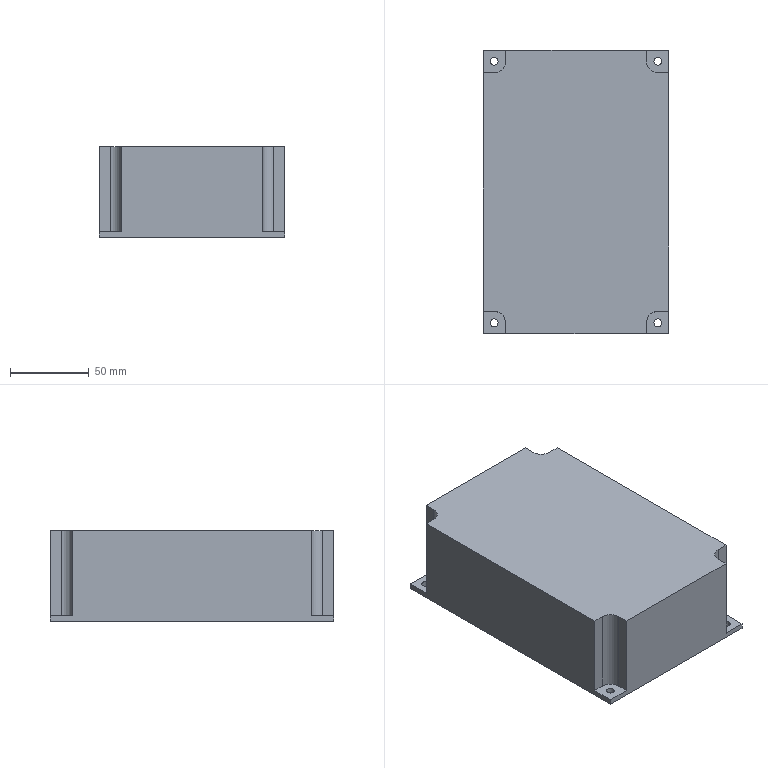Part | SolidWorks | features BaseBody 1 | 1 solid | 30 faces | box 118 x 180 x 57.5 mm | volume 1179222 mm3 | plane 18 | cylinder 12 | commonest cylinder face diameters 5 x8 14.547 x1 14.6 x1 14.623 x1 14.837 x1
STEP:
#1=CARTESIAN_POINT('',(194.55,-125.,1.5));
#2=VERTEX_POINT('',#1);
#3=CARTESIAN_POINT('',(189.55,-125.,1.5));
#4=VERTEX_POINT('',#3);
#5=CARTESIAN_POINT('',(192.05,-125.,1.5));
#6=DIRECTION('',(0.,0.,-1.));
#7=DIRECTION('',(-1.,0.,0.));
#8=AXIS2_PLACEMENT_3D('',#5,#6,#7);
#9=CIRCLE('',#8,2.5);
#10=EDGE_CURVE('',#2,#4,#9,.T.);
#11=ORIENTED_EDGE('',*,*,#10,.F.);
#12=CARTESIAN_POINT('',(194.55,-125.,-2.));
#13=VERTEX_POINT('',#12);
#14=CARTESIAN_POINT('',(194.55,-125.,101.5));
#15=DIRECTION('',(0.,0.,-1.));
#16=VECTOR('',#15,1000.);
#17=LINE('',#14,#16);
#18=EDGE_CURVE('',#2,#13,#17,.T.);
#19=ORIENTED_EDGE('',*,*,#18,.T.);
#20=CARTESIAN_POINT('',(189.55,-125.,-2.));
#21=VERTEX_POINT('',#20);
#22=CARTESIAN_POINT('',(192.05,-125.,-2.));
#23=DIRECTION('',(0.,0.,1.));
#24=DIRECTION('',(-1.,0.,0.));
#25=AXIS2_PLACEMENT_3D('',#22,#23,#24);
#26=CIRCLE('',#25,2.5);
#27=EDGE_CURVE('',#21,#13,#26,.T.);
#28=ORIENTED_EDGE('',*,*,#27,.F.);
#29=CARTESIAN_POINT('',(189.55,-125.,101.5));
#30=DIRECTION('',(0.,0.,-1.));
#31=VECTOR('',#30,1000.);
#32=LINE('',#29,#31);
#33=EDGE_CURVE('',#4,#21,#32,.T.);
#34=ORIENTED_EDGE('',*,*,#33,.F.);
#35=EDGE_LOOP('',(#11,#19,#28,#34));
#36=FACE_OUTER_BOUND('',#35,.T.);
#37=CARTESIAN_POINT('',(192.05,-125.,101.5));
#38=DIRECTION('',(0.,0.,-1.));
#39=DIRECTION('',(-1.,0.,0.));
#40=AXIS2_PLACEMENT_3D('',#37,#38,#39);
#41=CYLINDRICAL_SURFACE('',#40,2.5);
#42=ADVANCED_FACE('',(#36),#41,.F.);
#43=CARTESIAN_POINT('',(194.55,41.,1.5));
#44=VERTEX_POINT('',#43);
#45=CARTESIAN_POINT('',(189.55,41.,1.5));
#46=VERTEX_POINT('',#45);
#47=CARTESIAN_POINT('',(192.05,41.,1.5));
#48=DIRECTION('',(0.,0.,-1.));
#49=DIRECTION('',(-1.,0.,0.));
#50=AXIS2_PLACEMENT_3D('',#47,#48,#49);
#51=CIRCLE('',#50,2.5);
#52=EDGE_CURVE('',#44,#46,#51,.T.);
#53=ORIENTED_EDGE('',*,*,#52,.F.);
#54=CARTESIAN_POINT('',(194.55,41.,-2.));
#55=VERTEX_POINT('',#54);
#56=CARTESIAN_POINT('',(194.55,41.,101.5));
#57=DIRECTION('',(0.,0.,-1.));
#58=VECTOR('',#57,1000.);
#59=LINE('',#56,#58);
#60=EDGE_CURVE('',#44,#55,#59,.T.);
#61=ORIENTED_EDGE('',*,*,#60,.T.);
#62=CARTESIAN_POINT('',(189.55,41.,-2.));
#63=VERTEX_POINT('',#62);
#64=CARTESIAN_POINT('',(192.05,41.,-2.));
#65=DIRECTION('',(0.,0.,1.));
#66=DIRECTION('',(-1.,0.,0.));
#67=AXIS2_PLACEMENT_3D('',#64,#65,#66);
#68=CIRCLE('',#67,2.5);
#69=EDGE_CURVE('',#63,#55,#68,.T.);
#70=ORIENTED_EDGE('',*,*,#69,.F.);
#71=CARTESIAN_POINT('',(189.55,41.,101.5));
#72=DIRECTION('',(0.,0.,-1.));
#73=VECTOR('',#72,1000.);
#74=LINE('',#71,#73);
#75=EDGE_CURVE('',#46,#63,#74,.T.);
#76=ORIENTED_EDGE('',*,*,#75,.F.);
#77=EDGE_LOOP('',(#53,#61,#70,#76));
#78=FACE_OUTER_BOUND('',#77,.T.);
#79=CARTESIAN_POINT('',(192.05,41.,101.5));
#80=DIRECTION('',(0.,0.,-1.));
#81=DIRECTION('',(-1.,0.,0.));
#82=AXIS2_PLACEMENT_3D('',#79,#80,#81);
#83=CYLINDRICAL_SURFACE('',#82,2.5);
#84=ADVANCED_FACE('',(#78),#83,.F.);
#85=CARTESIAN_POINT('',(298.55,-125.,1.5));
#86=VERTEX_POINT('',#85);
#87=CARTESIAN_POINT('',(293.55,-125.,1.5));
#88=VERTEX_POINT('',#87);
#89=CARTESIAN_POINT('',(296.05,-125.,1.5));
#90=DIRECTION('',(0.,0.,-1.));
#91=DIRECTION('',(-1.,0.,0.));
#92=AXIS2_PLACEMENT_3D('',#89,#90,#91);
#93=CIRCLE('',#92,2.5);
#94=EDGE_CURVE('',#86,#88,#93,.T.);
#95=ORIENTED_EDGE('',*,*,#94,.F.);
#96=CARTESIAN_POINT('',(298.55,-125.,-2.));
#97=VERTEX_POINT('',#96);
#98=CARTESIAN_POINT('',(298.55,-125.,101.5));
#99=DIRECTION('',(0.,0.,-1.));
#100=VECTOR('',#99,1000.);
#101=LINE('',#98,#100);
#102=EDGE_CURVE('',#86,#97,#101,.T.);
#103=ORIENTED_EDGE('',*,*,#102,.T.);
#104=CARTESIAN_POINT('',(293.55,-125.,-2.));
#105=VERTEX_POINT('',#104);
#106=CARTESIAN_POINT('',(296.05,-125.,-2.));
#107=DIRECTION('',(0.,0.,1.));
#108=DIRECTION('',(-1.,0.,0.));
#109=AXIS2_PLACEMENT_3D('',#106,#107,#108);
#110=CIRCLE('',#109,2.5);
#111=EDGE_CURVE('',#105,#97,#110,.T.);
#112=ORIENTED_EDGE('',*,*,#111,.F.);
#113=CARTESIAN_POINT('',(293.55,-125.,101.5));
#114=DIRECTION('',(0.,0.,-1.));
#115=VECTOR('',#114,1000.);
#116=LINE('',#113,#115);
#117=EDGE_CURVE('',#88,#105,#116,.T.);
#118=ORIENTED_EDGE('',*,*,#117,.F.);
#119=EDGE_LOOP('',(#95,#103,#112,#118));
#120=FACE_OUTER_BOUND('',#119,.T.);
#121=CARTESIAN_POINT('',(296.05,-125.,101.5));
#122=DIRECTION('',(0.,0.,-1.));
#123=DIRECTION('',(-1.,0.,0.));
#124=AXIS2_PLACEMENT_3D('',#121,#122,#123);
#125=CYLINDRICAL_SURFACE('',#124,2.5);
#126=ADVANCED_FACE('',(#120),#125,.F.);
#127=CARTESIAN_POINT('',(298.55,41.,1.5));
#128=VERTEX_POINT('',#127);
#129=CARTESIAN_POINT('',(293.55,41.,1.5));
#130=VERTEX_POINT('',#129);
#131=CARTESIAN_POINT('',(296.05,41.,1.5));
#132=DIRECTION('',(0.,0.,-1.));
#133=DIRECTION('',(-1.,0.,0.));
#134=AXIS2_PLACEMENT_3D('',#131,#132,#133);
#135=CIRCLE('',#134,2.5);
#136=EDGE_CURVE('',#128,#130,#135,.T.);
#137=ORIENTED_EDGE('',*,*,#136,.F.);
#138=CARTESIAN_POINT('',(298.55,41.,-2.));
#139=VERTEX_POINT('',#138);
#140=CARTESIAN_POINT('',(298.55,41.,101.5));
#141=DIRECTION('',(0.,0.,-1.));
#142=VECTOR('',#141,1000.);
#143=LINE('',#140,#142);
#144=EDGE_CURVE('',#128,#139,#143,.T.);
#145=ORIENTED_EDGE('',*,*,#144,.T.);
#146=CARTESIAN_POINT('',(293.55,41.,-2.));
#147=VERTEX_POINT('',#146);
#148=CARTESIAN_POINT('',(296.05,41.,-2.));
#149=DIRECTION('',(0.,0.,1.));
#150=DIRECTION('',(-1.,0.,0.));
#151=AXIS2_PLACEMENT_3D('',#148,#149,#150);
#152=CIRCLE('',#151,2.5);
#153=EDGE_CURVE('',#147,#139,#152,.T.);
#154=ORIENTED_EDGE('',*,*,#153,.F.);
#155=CARTESIAN_POINT('',(293.55,41.,101.5));
#156=DIRECTION('',(0.,0.,-1.));
#157=VECTOR('',#156,1000.);
#158=LINE('',#155,#157);
#159=EDGE_CURVE('',#130,#147,#158,.T.);
#160=ORIENTED_EDGE('',*,*,#159,.F.);
#161=EDGE_LOOP('',(#137,#145,#154,#160));
#162=FACE_OUTER_BOUND('',#161,.T.);
#163=CARTESIAN_POINT('',(296.05,41.,101.5));
#164=DIRECTION('',(0.,0.,-1.));
#165=DIRECTION('',(-1.,0.,0.));
#166=AXIS2_PLACEMENT_3D('',#163,#164,#165);
#167=CYLINDRICAL_SURFACE('',#166,2.5);
#168=ADVANCED_FACE('',(#162),#167,.F.);
#169=CARTESIAN_POINT('',(192.05,33.581,1.5));
#170=VERTEX_POINT('',#169);
#171=CARTESIAN_POINT('',(199.469,41.,1.5));
#172=VERTEX_POINT('',#171);
#173=CARTESIAN_POINT('',(192.05,41.,1.5));
#174=DIRECTION('',(0.,0.,1.));
#175=DIRECTION('',(1.,0.,0.));
#176=AXIS2_PLACEMENT_3D('',#173,#174,#175);
#177=CIRCLE('',#176,7.419);
#178=EDGE_CURVE('',#170,#172,#177,.T.);
#179=ORIENTED_EDGE('',*,*,#178,.F.);
#180=CARTESIAN_POINT('',(192.05,33.581,55.5));
#181=VERTEX_POINT('',#180);
#182=CARTESIAN_POINT('',(192.05,33.581,1.5));
#183=DIRECTION('',(0.,0.,-1.));
#184=VECTOR('',#183,1000.);
#185=LINE('',#182,#184);
#186=EDGE_CURVE('',#181,#170,#185,.T.);
#187=ORIENTED_EDGE('',*,*,#186,.F.);
#188=CARTESIAN_POINT('',(199.469,41.,55.5));
#189=VERTEX_POINT('',#188);
#190=CARTESIAN_POINT('',(192.05,41.,55.5));
#191=DIRECTION('',(0.,0.,1.));
#192=DIRECTION('',(1.,0.,0.));
#193=AXIS2_PLACEMENT_3D('',#190,#191,#192);
#194=CIRCLE('',#193,7.419);
#195=EDGE_CURVE('',#181,#189,#194,.T.);
#196=ORIENTED_EDGE('',*,*,#195,.T.);
#197=CARTESIAN_POINT('',(199.469,41.,1.5));
#198=DIRECTION('',(0.,0.,1.));
#199=VECTOR('',#198,1000.);
#200=LINE('',#197,#199);
#201=EDGE_CURVE('',#172,#189,#200,.T.);
#202=ORIENTED_EDGE('',*,*,#201,.F.);
#203=EDGE_LOOP('',(#179,#187,#196,#202));
#204=FACE_OUTER_BOUND('',#203,.T.);
#205=CARTESIAN_POINT('',(192.05,41.,1.5));
#206=DIRECTION('',(0.,0.,1.));
#207=DIRECTION('',(1.,0.,0.));
#208=AXIS2_PLACEMENT_3D('',#205,#206,#207);
#209=CYLINDRICAL_SURFACE('',#208,7.419);
#210=ADVANCED_FACE('',(#204),#209,.F.);
#211=CARTESIAN_POINT('',(296.05,-117.7,1.5));
#212=VERTEX_POINT('',#211);
#213=CARTESIAN_POINT('',(288.75,-125.,1.5));
#214=VERTEX_POINT('',#213);
#215=CARTESIAN_POINT('',(296.05,-125.,1.5));
#216=DIRECTION('',(0.,0.,1.));
#217=DIRECTION('',(1.,0.,0.));
#218=AXIS2_PLACEMENT_3D('',#215,#216,#217);
#219=CIRCLE('',#218,7.3);
#220=EDGE_CURVE('',#212,#214,#219,.T.);
#221=ORIENTED_EDGE('',*,*,#220,.F.);
#222=CARTESIAN_POINT('',(296.05,-117.7,55.5));
#223=VERTEX_POINT('',#222);
#224=CARTESIAN_POINT('',(296.05,-117.7,1.5));
#225=DIRECTION('',(0.,0.,-1.));
#226=VECTOR('',#225,1000.);
#227=LINE('',#224,#226);
#228=EDGE_CURVE('',#223,#212,#227,.T.);
#229=ORIENTED_EDGE('',*,*,#228,.F.);
#230=CARTESIAN_POINT('',(288.75,-125.,55.5));
#231=VERTEX_POINT('',#230);
#232=CARTESIAN_POINT('',(296.05,-125.,55.5));
#233=DIRECTION('',(0.,0.,1.));
#234=DIRECTION('',(1.,0.,0.));
#235=AXIS2_PLACEMENT_3D('',#232,#233,#234);
#236=CIRCLE('',#235,7.3);
#237=EDGE_CURVE('',#223,#231,#236,.T.);
#238=ORIENTED_EDGE('',*,*,#237,.T.);
#239=CARTESIAN_POINT('',(288.75,-125.,1.5));
#240=DIRECTION('',(0.,0.,1.));
#241=VECTOR('',#240,1000.);
#242=LINE('',#239,#241);
#243=EDGE_CURVE('',#214,#231,#242,.T.);
#244=ORIENTED_EDGE('',*,*,#243,.F.);
#245=EDGE_LOOP('',(#221,#229,#238,#244));
#246=FACE_OUTER_BOUND('',#245,.T.);
#247=CARTESIAN_POINT('',(296.05,-125.,1.5));
#248=DIRECTION('',(0.,0.,1.));
#249=DIRECTION('',(1.,0.,0.));
#250=AXIS2_PLACEMENT_3D('',#247,#248,#249);
#251=CYLINDRICAL_SURFACE('',#250,7.3);
#252=ADVANCED_FACE('',(#246),#251,.F.);
#253=CARTESIAN_POINT('',(199.361,-125.,1.5));
#254=VERTEX_POINT('',#253);
#255=CARTESIAN_POINT('',(192.05,-117.689,1.5));
#256=VERTEX_POINT('',#255);
#257=CARTESIAN_POINT('',(192.05,-125.,1.5));
#258=DIRECTION('',(0.,0.,1.));
#259=DIRECTION('',(1.,0.,0.));
#260=AXIS2_PLACEMENT_3D('',#257,#258,#259);
#261=CIRCLE('',#260,7.311);
#262=EDGE_CURVE('',#254,#256,#261,.T.);
#263=ORIENTED_EDGE('',*,*,#262,.F.);
#264=CARTESIAN_POINT('',(199.361,-125.,55.5));
#265=VERTEX_POINT('',#264);
#266=CARTESIAN_POINT('',(199.361,-125.,1.5));
#267=DIRECTION('',(0.,0.,-1.));
#268=VECTOR('',#267,1000.);
#269=LINE('',#266,#268);
#270=EDGE_CURVE('',#265,#254,#269,.T.);
#271=ORIENTED_EDGE('',*,*,#270,.F.);
#272=CARTESIAN_POINT('',(192.05,-117.689,55.5));
#273=VERTEX_POINT('',#272);
#274=CARTESIAN_POINT('',(192.05,-125.,55.5));
#275=DIRECTION('',(0.,0.,1.));
#276=DIRECTION('',(1.,0.,0.));
#277=AXIS2_PLACEMENT_3D('',#274,#275,#276);
#278=CIRCLE('',#277,7.311);
#279=EDGE_CURVE('',#265,#273,#278,.T.);
#280=ORIENTED_EDGE('',*,*,#279,.T.);
#281=CARTESIAN_POINT('',(192.05,-117.689,1.5));
#282=DIRECTION('',(0.,0.,1.));
#283=VECTOR('',#282,1000.);
#284=LINE('',#281,#283);
#285=EDGE_CURVE('',#256,#273,#284,.T.);
#286=ORIENTED_EDGE('',*,*,#285,.F.);
#287=EDGE_LOOP('',(#263,#271,#280,#286));
#288=FACE_OUTER_BOUND('',#287,.T.);
#289=CARTESIAN_POINT('',(192.05,-125.,1.5));
#290=DIRECTION('',(0.,0.,1.));
#291=DIRECTION('',(1.,0.,0.));
#292=AXIS2_PLACEMENT_3D('',#289,#290,#291);
#293=CYLINDRICAL_SURFACE('',#292,7.311);
#294=ADVANCED_FACE('',(#288),#293,.F.);
#295=CARTESIAN_POINT('',(288.795,40.489,1.5));
#296=VERTEX_POINT('',#295);
#297=CARTESIAN_POINT('',(288.795,40.489,55.5));
#298=VERTEX_POINT('',#297);
#299=CARTESIAN_POINT('',(288.795,40.489,1.5));
#300=DIRECTION('',(0.,0.,1.));
#301=VECTOR('',#300,1000.);
#302=LINE('',#299,#301);
#303=EDGE_CURVE('',#296,#298,#302,.T.);
#304=ORIENTED_EDGE('',*,*,#303,.T.);
#305=CARTESIAN_POINT('',(294.989,33.805,55.5));
#306=VERTEX_POINT('',#305);
#307=CARTESIAN_POINT('',(296.05,41.,55.5));
#308=DIRECTION('',(0.,0.,1.));
#309=DIRECTION('',(1.,0.,0.));
#310=AXIS2_PLACEMENT_3D('',#307,#308,#309);
#311=CIRCLE('',#310,7.273);
#312=EDGE_CURVE('',#298,#306,#311,.T.);
#313=ORIENTED_EDGE('',*,*,#312,.T.);
#314=CARTESIAN_POINT('',(294.989,33.805,1.5));
#315=VERTEX_POINT('',#314);
#316=CARTESIAN_POINT('',(294.989,33.805,1.5));
#317=DIRECTION('',(0.,0.,-1.));
#318=VECTOR('',#317,1000.);
#319=LINE('',#316,#318);
#320=EDGE_CURVE('',#306,#315,#319,.T.);
#321=ORIENTED_EDGE('',*,*,#320,.T.);
#322=CARTESIAN_POINT('',(296.05,41.,1.5));
#323=DIRECTION('',(0.,0.,1.));
#324=DIRECTION('',(1.,0.,0.));
#325=AXIS2_PLACEMENT_3D('',#322,#323,#324);
#326=CIRCLE('',#325,7.273);
#327=EDGE_CURVE('',#296,#315,#326,.T.);
#328=ORIENTED_EDGE('',*,*,#327,.F.);
#329=EDGE_LOOP('',(#304,#313,#321,#328));
#330=FACE_OUTER_BOUND('',#329,.T.);
#331=CARTESIAN_POINT('',(296.05,41.,1.5));
#332=DIRECTION('',(0.,0.,1.));
#333=DIRECTION('',(1.,0.,0.));
#334=AXIS2_PLACEMENT_3D('',#331,#332,#333);
#335=CYLINDRICAL_SURFACE('',#334,7.273);
#336=ADVANCED_FACE('',(#330),#335,.F.);
#337=CARTESIAN_POINT('',(199.361,-132.,55.5));
#338=VERTEX_POINT('',#337);
#339=CARTESIAN_POINT('',(199.361,-36.,55.5));
#340=DIRECTION('',(0.,1.,0.));
#341=VECTOR('',#340,1000.);
#342=LINE('',#339,#341);
#343=EDGE_CURVE('',#338,#265,#342,.T.);
#344=ORIENTED_EDGE('',*,*,#343,.T.);
#345=ORIENTED_EDGE('',*,*,#270,.T.);
#346=CARTESIAN_POINT('',(199.361,-132.,1.5));
#347=VERTEX_POINT('',#346);
#348=CARTESIAN_POINT('',(199.361,-126.219,1.5));
#349=DIRECTION('',(0.,1.,0.));
#350=VECTOR('',#349,1000.);
#351=LINE('',#348,#350);
#352=EDGE_CURVE('',#347,#254,#351,.T.);
#353=ORIENTED_EDGE('',*,*,#352,.F.);
#354=CARTESIAN_POINT('',(199.361,-132.,-2.));
#355=DIRECTION('',(0.,0.,1.));
#356=VECTOR('',#355,1000.);
#357=LINE('',#354,#356);
#358=EDGE_CURVE('',#347,#338,#357,.T.);
#359=ORIENTED_EDGE('',*,*,#358,.T.);
#360=EDGE_LOOP('',(#344,#345,#353,#359));
#361=FACE_OUTER_BOUND('',#360,.T.);
#362=CARTESIAN_POINT('',(199.361,-134.75,1.5));
#363=DIRECTION('',(-1.,0.,0.));
#364=DIRECTION('',(0.,0.,1.));
#365=AXIS2_PLACEMENT_3D('',#362,#363,#364);
#366=PLANE('',#365);
#367=ADVANCED_FACE('',(#361),#366,.T.);
#368=CARTESIAN_POINT('',(288.75,-132.,55.5));
#369=VERTEX_POINT('',#368);
#370=CARTESIAN_POINT('',(288.75,-36.,55.5));
#371=DIRECTION('',(0.,-1.,0.));
#372=VECTOR('',#371,1000.);
#373=LINE('',#370,#372);
#374=EDGE_CURVE('',#231,#369,#373,.T.);
#375=ORIENTED_EDGE('',*,*,#374,.T.);
#376=CARTESIAN_POINT('',(288.75,-132.,1.5));
#377=VERTEX_POINT('',#376);
#378=CARTESIAN_POINT('',(288.75,-132.,-2.));
#379=DIRECTION('',(0.,0.,-1.));
#380=VECTOR('',#379,1000.);
#381=LINE('',#378,#380);
#382=EDGE_CURVE('',#369,#377,#381,.T.);
#383=ORIENTED_EDGE('',*,*,#382,.T.);
#384=CARTESIAN_POINT('',(288.75,-126.219,1.5));
#385=DIRECTION('',(0.,-1.,0.));
#386=VECTOR('',#385,1000.);
#387=LINE('',#384,#386);
#388=EDGE_CURVE('',#214,#377,#387,.T.);
#389=ORIENTED_EDGE('',*,*,#388,.F.);
#390=ORIENTED_EDGE('',*,*,#243,.T.);
#391=EDGE_LOOP('',(#375,#383,#389,#390));
#392=FACE_OUTER_BOUND('',#391,.T.);
#393=CARTESIAN_POINT('',(288.75,-125.,1.5));
#394=DIRECTION('',(1.,0.,0.));
#395=DIRECTION('',(0.,0.,1.));
#396=AXIS2_PLACEMENT_3D('',#393,#394,#395);
#397=PLANE('',#396);
#398=ADVANCED_FACE('',(#392),#397,.T.);
#399=CARTESIAN_POINT('',(185.05,33.581,55.5));
#400=VERTEX_POINT('',#399);
#401=CARTESIAN_POINT('',(-87.05,33.581,55.5));
#402=DIRECTION('',(1.,0.,0.));
#403=VECTOR('',#402,1000.);
#404=LINE('',#401,#403);
#405=EDGE_CURVE('',#400,#181,#404,.T.);
#406=ORIENTED_EDGE('',*,*,#405,.T.);
#407=ORIENTED_EDGE('',*,*,#186,.T.);
#408=CARTESIAN_POINT('',(185.05,33.581,1.5));
#409=VERTEX_POINT('',#408);
#410=CARTESIAN_POINT('',(192.296,33.581,1.5));
#411=DIRECTION('',(1.,0.,0.));
#412=VECTOR('',#411,1000.);
#413=LINE('',#410,#412);
#414=EDGE_CURVE('',#409,#170,#413,.T.);
#415=ORIENTED_EDGE('',*,*,#414,.F.);
#416=CARTESIAN_POINT('',(185.05,33.581,6.));
#417=DIRECTION('',(0.,0.,1.));
#418=VECTOR('',#417,1000.);
#419=LINE('',#416,#418);
#420=EDGE_CURVE('',#409,#400,#419,.T.);
#421=ORIENTED_EDGE('',*,*,#420,.T.);
#422=EDGE_LOOP('',(#406,#407,#415,#421));
#423=FACE_OUTER_BOUND('',#422,.T.);
#424=CARTESIAN_POINT('',(184.8,33.581,1.5));
#425=DIRECTION('',(0.,1.,0.));
#426=DIRECTION('',(1.,0.,0.));
#427=AXIS2_PLACEMENT_3D('',#424,#425,#426);
#428=PLANE('',#427);
#429=ADVANCED_FACE('',(#423),#428,.T.);
#430=CARTESIAN_POINT('',(185.05,-117.689,55.5));
#431=VERTEX_POINT('',#430);
#432=CARTESIAN_POINT('',(-87.05,-117.689,55.5));
#433=DIRECTION('',(-1.,0.,0.));
#434=VECTOR('',#433,1000.);
#435=LINE('',#432,#434);
#436=EDGE_CURVE('',#273,#431,#435,.T.);
#437=ORIENTED_EDGE('',*,*,#436,.T.);
#438=CARTESIAN_POINT('',(185.05,-117.689,1.5));
#439=VERTEX_POINT('',#438);
#440=CARTESIAN_POINT('',(185.05,-117.689,6.));
#441=DIRECTION('',(0.,0.,-1.));
#442=VECTOR('',#441,1000.);
#443=LINE('',#440,#442);
#444=EDGE_CURVE('',#431,#439,#443,.T.);
#445=ORIENTED_EDGE('',*,*,#444,.T.);
#446=CARTESIAN_POINT('',(192.296,-117.689,1.5));
#447=DIRECTION('',(-1.,0.,0.));
#448=VECTOR('',#447,1000.);
#449=LINE('',#446,#448);
#450=EDGE_CURVE('',#256,#439,#449,.T.);
#451=ORIENTED_EDGE('',*,*,#450,.F.);
#452=ORIENTED_EDGE('',*,*,#285,.T.);
#453=EDGE_LOOP('',(#437,#445,#451,#452));
#454=FACE_OUTER_BOUND('',#453,.T.);
#455=CARTESIAN_POINT('',(192.05,-117.689,1.5));
#456=DIRECTION('',(0.,-1.,0.));
#457=DIRECTION('',(0.,0.,-1.));
#458=AXIS2_PLACEMENT_3D('',#455,#456,#457);
#459=PLANE('',#458);
#460=ADVANCED_FACE('',(#454),#459,.T.);
#461=CARTESIAN_POINT('',(192.05,-125.,1.5));
#462=DIRECTION('',(0.,0.,-1.));
#463=DIRECTION('',(-1.,0.,0.));
#464=AXIS2_PLACEMENT_3D('',#461,#462,#463);
#465=CIRCLE('',#464,2.5);
#466=EDGE_CURVE('',#4,#2,#465,.T.);
#467=ORIENTED_EDGE('',*,*,#466,.T.);
#468=ORIENTED_EDGE('',*,*,#10,.T.);
#469=EDGE_LOOP('',(#467,#468));
#470=FACE_BOUND('',#469,.T.);
#471=ORIENTED_EDGE('',*,*,#352,.T.);
#472=ORIENTED_EDGE('',*,*,#262,.T.);
#473=ORIENTED_EDGE('',*,*,#450,.T.);
#474=CARTESIAN_POINT('',(185.05,-132.,1.5));
#475=VERTEX_POINT('',#474);
#476=CARTESIAN_POINT('',(185.05,66.5,1.5));
#477=DIRECTION('',(0.,-1.,0.));
#478=VECTOR('',#477,1000.);
#479=LINE('',#476,#478);
#480=EDGE_CURVE('',#439,#475,#479,.T.);
#481=ORIENTED_EDGE('',*,*,#480,.T.);
#482=CARTESIAN_POINT('',(303.05,-132.,1.5));
#483=DIRECTION('',(1.,0.,0.));
#484=VECTOR('',#483,1000.);
#485=LINE('',#482,#484);
#486=EDGE_CURVE('',#475,#347,#485,.T.);
#487=ORIENTED_EDGE('',*,*,#486,.T.);
#488=EDGE_LOOP('',(#471,#472,#473,#481,#487));
#489=FACE_OUTER_BOUND('',#488,.T.);
#490=CARTESIAN_POINT('',(192.296,-126.219,1.5));
#491=DIRECTION('',(0.,0.,1.));
#492=DIRECTION('',(1.,0.,0.));
#493=AXIS2_PLACEMENT_3D('',#490,#491,#492);
#494=PLANE('',#493);
#495=ADVANCED_FACE('',(#470,#489),#494,.T.);
#496=CARTESIAN_POINT('',(288.795,48.,55.5));
#497=VERTEX_POINT('',#496);
#498=CARTESIAN_POINT('',(288.795,48.,1.5));
#499=VERTEX_POINT('',#498);
#500=CARTESIAN_POINT('',(288.795,48.,-2.));
#501=DIRECTION('',(0.,0.,-1.));
#502=VECTOR('',#501,1000.);
#503=LINE('',#500,#502);
#504=EDGE_CURVE('',#497,#499,#503,.T.);
#505=ORIENTED_EDGE('',*,*,#504,.F.);
#506=CARTESIAN_POINT('',(288.795,-36.,55.5));
#507=DIRECTION('',(0.,-1.,0.));
#508=VECTOR('',#507,1000.);
#509=LINE('',#506,#508);
#510=EDGE_CURVE('',#497,#298,#509,.T.);
#511=ORIENTED_EDGE('',*,*,#510,.T.);
#512=ORIENTED_EDGE('',*,*,#303,.F.);
#513=CARTESIAN_POINT('',(288.795,-126.219,1.5));
#514=DIRECTION('',(0.,-1.,0.));
#515=VECTOR('',#514,1000.);
#516=LINE('',#513,#515);
#517=EDGE_CURVE('',#499,#296,#516,.T.);
#518=ORIENTED_EDGE('',*,*,#517,.F.);
#519=EDGE_LOOP('',(#505,#511,#512,#518));
#520=FACE_OUTER_BOUND('',#519,.T.);
#521=CARTESIAN_POINT('',(288.795,40.489,1.5));
#522=DIRECTION('',(-1.,0.,0.));
#523=DIRECTION('',(0.,0.,1.));
#524=AXIS2_PLACEMENT_3D('',#521,#522,#523);
#525=PLANE('',#524);
#526=ADVANCED_FACE('',(#520),#525,.F.);
#527=CARTESIAN_POINT('',(192.05,41.,1.5));
#528=DIRECTION('',(0.,0.,-1.));
#529=DIRECTION('',(-1.,0.,0.));
#530=AXIS2_PLACEMENT_3D('',#527,#528,#529);
#531=CIRCLE('',#530,2.5);
#532=EDGE_CURVE('',#46,#44,#531,.T.);
#533=ORIENTED_EDGE('',*,*,#532,.T.);
#534=ORIENTED_EDGE('',*,*,#52,.T.);
#535=EDGE_LOOP('',(#533,#534));
#536=FACE_BOUND('',#535,.T.);
#537=ORIENTED_EDGE('',*,*,#414,.T.);
#538=ORIENTED_EDGE('',*,*,#178,.T.);
#539=CARTESIAN_POINT('',(199.469,48.,1.5));
#540=VERTEX_POINT('',#539);
#541=CARTESIAN_POINT('',(199.469,41.,1.5));
#542=DIRECTION('',(0.,-1.,0.));
#543=VECTOR('',#542,1000.);
#544=LINE('',#541,#543);
#545=EDGE_CURVE('',#540,#172,#544,.T.);
#546=ORIENTED_EDGE('',*,*,#545,.F.);
#547=CARTESIAN_POINT('',(185.05,48.,1.5));
#548=VERTEX_POINT('',#547);
#549=CARTESIAN_POINT('',(325.05,48.,1.5));
#550=DIRECTION('',(1.,0.,0.));
#551=VECTOR('',#550,1000.);
#552=LINE('',#549,#551);
#553=EDGE_CURVE('',#548,#540,#552,.T.);
#554=ORIENTED_EDGE('',*,*,#553,.F.);
#555=CARTESIAN_POINT('',(185.05,66.5,1.5));
#556=DIRECTION('',(0.,-1.,0.));
#557=VECTOR('',#556,1000.);
#558=LINE('',#555,#557);
#559=EDGE_CURVE('',#548,#409,#558,.T.);
#560=ORIENTED_EDGE('',*,*,#559,.T.);
#561=EDGE_LOOP('',(#537,#538,#546,#554,#560));
#562=FACE_OUTER_BOUND('',#561,.T.);
#563=CARTESIAN_POINT('',(192.296,-126.219,1.5));
#564=DIRECTION('',(0.,0.,1.));
#565=DIRECTION('',(1.,0.,0.));
#566=AXIS2_PLACEMENT_3D('',#563,#564,#565);
#567=PLANE('',#566);
#568=ADVANCED_FACE('',(#536,#562),#567,.T.);
#569=CARTESIAN_POINT('',(199.469,48.,55.5));
#570=VERTEX_POINT('',#569);
#571=CARTESIAN_POINT('',(199.469,-36.,55.5));
#572=DIRECTION('',(0.,1.,0.));
#573=VECTOR('',#572,1000.);
#574=LINE('',#571,#573);
#575=EDGE_CURVE('',#189,#570,#574,.T.);
#576=ORIENTED_EDGE('',*,*,#575,.T.);
#577=CARTESIAN_POINT('',(199.469,48.,-2.));
#578=DIRECTION('',(0.,0.,1.));
#579=VECTOR('',#578,1000.);
#580=LINE('',#577,#579);
#581=EDGE_CURVE('',#540,#570,#580,.T.);
#582=ORIENTED_EDGE('',*,*,#581,.F.);
#583=ORIENTED_EDGE('',*,*,#545,.T.);
#584=ORIENTED_EDGE('',*,*,#201,.T.);
#585=EDGE_LOOP('',(#576,#582,#583,#584));
#586=FACE_OUTER_BOUND('',#585,.T.);
#587=CARTESIAN_POINT('',(199.469,41.,1.5));
#588=DIRECTION('',(-1.,0.,0.));
#589=DIRECTION('',(0.,0.,1.));
#590=AXIS2_PLACEMENT_3D('',#587,#588,#589);
#591=PLANE('',#590);
#592=ADVANCED_FACE('',(#586),#591,.T.);
#593=CARTESIAN_POINT('',(296.05,-125.,1.5));
#594=DIRECTION('',(0.,0.,-1.));
#595=DIRECTION('',(-1.,0.,0.));
#596=AXIS2_PLACEMENT_3D('',#593,#594,#595);
#597=CIRCLE('',#596,2.5);
#598=EDGE_CURVE('',#88,#86,#597,.T.);
#599=ORIENTED_EDGE('',*,*,#598,.T.);
#600=ORIENTED_EDGE('',*,*,#94,.T.);
#601=EDGE_LOOP('',(#599,#600));
#602=FACE_BOUND('',#601,.T.);
#603=CARTESIAN_POINT('',(303.05,-117.7,1.5));
#604=VERTEX_POINT('',#603);
#605=CARTESIAN_POINT('',(303.3,-117.7,1.5));
#606=DIRECTION('',(1.,0.,0.));
#607=VECTOR('',#606,1000.);
#608=LINE('',#605,#607);
#609=EDGE_CURVE('',#212,#604,#608,.T.);
#610=ORIENTED_EDGE('',*,*,#609,.F.);
#611=ORIENTED_EDGE('',*,*,#220,.T.);
#612=ORIENTED_EDGE('',*,*,#388,.T.);
#613=CARTESIAN_POINT('',(303.05,-132.,1.5));
#614=VERTEX_POINT('',#613);
#615=CARTESIAN_POINT('',(303.05,-132.,1.5));
#616=DIRECTION('',(1.,0.,0.));
#617=VECTOR('',#616,1000.);
#618=LINE('',#615,#617);
#619=EDGE_CURVE('',#377,#614,#618,.T.);
#620=ORIENTED_EDGE('',*,*,#619,.T.);
#621=CARTESIAN_POINT('',(303.05,-40.,1.5));
#622=DIRECTION('',(0.,1.,0.));
#623=VECTOR('',#622,1000.);
#624=LINE('',#621,#623);
#625=EDGE_CURVE('',#614,#604,#624,.T.);
#626=ORIENTED_EDGE('',*,*,#625,.T.);
#627=EDGE_LOOP('',(#610,#611,#612,#620,#626));
#628=FACE_OUTER_BOUND('',#627,.T.);
#629=CARTESIAN_POINT('',(192.296,-126.219,1.5));
#630=DIRECTION('',(0.,0.,1.));
#631=DIRECTION('',(1.,0.,0.));
#632=AXIS2_PLACEMENT_3D('',#629,#630,#631);
#633=PLANE('',#632);
#634=ADVANCED_FACE('',(#602,#628),#633,.T.);
#635=CARTESIAN_POINT('',(303.05,-117.7,55.5));
#636=VERTEX_POINT('',#635);
#637=CARTESIAN_POINT('',(-87.05,-117.7,55.5));
#638=DIRECTION('',(-1.,0.,0.));
#639=VECTOR('',#638,1000.);
#640=LINE('',#637,#639);
#641=EDGE_CURVE('',#636,#223,#640,.T.);
#642=ORIENTED_EDGE('',*,*,#641,.T.);
#643=ORIENTED_EDGE('',*,*,#228,.T.);
#644=ORIENTED_EDGE('',*,*,#609,.T.);
#645=CARTESIAN_POINT('',(303.05,-117.7,6.));
#646=DIRECTION('',(0.,0.,1.));
#647=VECTOR('',#646,1000.);
#648=LINE('',#645,#647);
#649=EDGE_CURVE('',#604,#636,#648,.T.);
#650=ORIENTED_EDGE('',*,*,#649,.T.);
#651=EDGE_LOOP('',(#642,#643,#644,#650));
#652=FACE_OUTER_BOUND('',#651,.T.);
#653=CARTESIAN_POINT('',(303.3,-117.7,1.5));
#654=DIRECTION('',(0.,-1.,0.));
#655=DIRECTION('',(0.,0.,-1.));
#656=AXIS2_PLACEMENT_3D('',#653,#654,#655);
#657=PLANE('',#656);
#658=ADVANCED_FACE('',(#652),#657,.T.);
#659=ORIENTED_EDGE('',*,*,#436,.F.);
#660=ORIENTED_EDGE('',*,*,#279,.F.);
#661=ORIENTED_EDGE('',*,*,#343,.F.);
#662=CARTESIAN_POINT('',(303.05,-132.,55.5));
#663=DIRECTION('',(1.,0.,0.));
#664=VECTOR('',#663,1000.);
#665=LINE('',#662,#664);
#666=EDGE_CURVE('',#338,#369,#665,.T.);
#667=ORIENTED_EDGE('',*,*,#666,.T.);
#668=ORIENTED_EDGE('',*,*,#374,.F.);
#669=ORIENTED_EDGE('',*,*,#237,.F.);
#670=ORIENTED_EDGE('',*,*,#641,.F.);
#671=CARTESIAN_POINT('',(303.05,33.805,55.5));
#672=VERTEX_POINT('',#671);
#673=CARTESIAN_POINT('',(303.05,-40.,55.5));
#674=DIRECTION('',(0.,1.,0.));
#675=VECTOR('',#674,1000.);
#676=LINE('',#673,#675);
#677=EDGE_CURVE('',#636,#672,#676,.T.);
#678=ORIENTED_EDGE('',*,*,#677,.T.);
#679=CARTESIAN_POINT('',(303.3,33.805,55.5));
#680=DIRECTION('',(-1.,0.,0.));
#681=VECTOR('',#680,1000.);
#682=LINE('',#679,#681);
#683=EDGE_CURVE('',#672,#306,#682,.T.);
#684=ORIENTED_EDGE('',*,*,#683,.T.);
#685=ORIENTED_EDGE('',*,*,#312,.F.);
#686=ORIENTED_EDGE('',*,*,#510,.F.);
#687=CARTESIAN_POINT('',(325.05,48.,55.5));
#688=DIRECTION('',(1.,0.,0.));
#689=VECTOR('',#688,1000.);
#690=LINE('',#687,#689);
#691=EDGE_CURVE('',#570,#497,#690,.T.);
#692=ORIENTED_EDGE('',*,*,#691,.F.);
#693=ORIENTED_EDGE('',*,*,#575,.F.);
#694=ORIENTED_EDGE('',*,*,#195,.F.);
#695=ORIENTED_EDGE('',*,*,#405,.F.);
#696=CARTESIAN_POINT('',(185.05,66.5,55.5));
#697=DIRECTION('',(0.,-1.,0.));
#698=VECTOR('',#697,1000.);
#699=LINE('',#696,#698);
#700=EDGE_CURVE('',#400,#431,#699,.T.);
#701=ORIENTED_EDGE('',*,*,#700,.T.);
#702=EDGE_LOOP('',(#659,#660,#661,#667,#668,#669,#670,#678,#684,#685,#686,#692,#693,#694,#695,#701));
#703=FACE_OUTER_BOUND('',#702,.T.);
#704=CARTESIAN_POINT('',(-87.05,-36.,55.5));
#705=DIRECTION('',(0.,0.,-1.));
#706=DIRECTION('',(0.,-1.,0.));
#707=AXIS2_PLACEMENT_3D('',#704,#705,#706);
#708=PLANE('',#707);
#709=ADVANCED_FACE('',(#703),#708,.F.);
#710=ORIENTED_EDGE('',*,*,#320,.F.);
#711=ORIENTED_EDGE('',*,*,#683,.F.);
#712=CARTESIAN_POINT('',(303.05,33.805,1.5));
#713=VERTEX_POINT('',#712);
#714=CARTESIAN_POINT('',(303.05,33.805,6.));
#715=DIRECTION('',(0.,0.,-1.));
#716=VECTOR('',#715,1000.);
#717=LINE('',#714,#716);
#718=EDGE_CURVE('',#672,#713,#717,.T.);
#719=ORIENTED_EDGE('',*,*,#718,.T.);
#720=CARTESIAN_POINT('',(192.296,33.805,1.5));
#721=DIRECTION('',(1.,0.,0.));
#722=VECTOR('',#721,1000.);
#723=LINE('',#720,#722);
#724=EDGE_CURVE('',#315,#713,#723,.T.);
#725=ORIENTED_EDGE('',*,*,#724,.F.);
#726=EDGE_LOOP('',(#710,#711,#719,#725));
#727=FACE_OUTER_BOUND('',#726,.T.);
#728=CARTESIAN_POINT('',(303.3,33.805,1.5));
#729=DIRECTION('',(0.,-1.,0.));
#730=DIRECTION('',(-1.,0.,0.));
#731=AXIS2_PLACEMENT_3D('',#728,#729,#730);
#732=PLANE('',#731);
#733=ADVANCED_FACE('',(#727),#732,.F.);
#734=CARTESIAN_POINT('',(296.05,41.,1.5));
#735=DIRECTION('',(0.,0.,-1.));
#736=DIRECTION('',(-1.,0.,0.));
#737=AXIS2_PLACEMENT_3D('',#734,#735,#736);
#738=CIRCLE('',#737,2.5);
#739=EDGE_CURVE('',#130,#128,#738,.T.);
#740=ORIENTED_EDGE('',*,*,#739,.T.);
#741=ORIENTED_EDGE('',*,*,#136,.T.);
#742=EDGE_LOOP('',(#740,#741));
#743=FACE_BOUND('',#742,.T.);
#744=ORIENTED_EDGE('',*,*,#327,.T.);
#745=ORIENTED_EDGE('',*,*,#724,.T.);
#746=CARTESIAN_POINT('',(303.05,48.,1.5));
#747=VERTEX_POINT('',#746);
#748=CARTESIAN_POINT('',(303.05,-40.,1.5));
#749=DIRECTION('',(0.,1.,0.));
#750=VECTOR('',#749,1000.);
#751=LINE('',#748,#750);
#752=EDGE_CURVE('',#713,#747,#751,.T.);
#753=ORIENTED_EDGE('',*,*,#752,.T.);
#754=CARTESIAN_POINT('',(325.05,48.,1.5));
#755=DIRECTION('',(1.,0.,0.));
#756=VECTOR('',#755,1000.);
#757=LINE('',#754,#756);
#758=EDGE_CURVE('',#499,#747,#757,.T.);
#759=ORIENTED_EDGE('',*,*,#758,.F.);
#760=ORIENTED_EDGE('',*,*,#517,.T.);
#761=EDGE_LOOP('',(#744,#745,#753,#759,#760));
#762=FACE_OUTER_BOUND('',#761,.T.);
#763=CARTESIAN_POINT('',(192.296,-126.219,1.5));
#764=DIRECTION('',(0.,0.,1.));
#765=DIRECTION('',(1.,0.,0.));
#766=AXIS2_PLACEMENT_3D('',#763,#764,#765);
#767=PLANE('',#766);
#768=ADVANCED_FACE('',(#743,#762),#767,.T.);
#769=CARTESIAN_POINT('',(303.05,-132.,-2.));
#770=VERTEX_POINT('',#769);
#771=CARTESIAN_POINT('',(303.05,-132.,6.));
#772=DIRECTION('',(0.,0.,1.));
#773=VECTOR('',#772,1000.);
#774=LINE('',#771,#773);
#775=EDGE_CURVE('',#770,#614,#774,.T.);
#776=ORIENTED_EDGE('',*,*,#775,.T.);
#777=ORIENTED_EDGE('',*,*,#619,.F.);
#778=ORIENTED_EDGE('',*,*,#382,.F.);
#779=ORIENTED_EDGE('',*,*,#666,.F.);
#780=ORIENTED_EDGE('',*,*,#358,.F.);
#781=ORIENTED_EDGE('',*,*,#486,.F.);
#782=CARTESIAN_POINT('',(185.05,-132.,-2.));
#783=VERTEX_POINT('',#782);
#784=CARTESIAN_POINT('',(185.05,-132.,6.));
#785=DIRECTION('',(0.,0.,-1.));
#786=VECTOR('',#785,1000.);
#787=LINE('',#784,#786);
#788=EDGE_CURVE('',#475,#783,#787,.T.);
#789=ORIENTED_EDGE('',*,*,#788,.T.);
#790=CARTESIAN_POINT('',(-87.05,-132.,-2.));
#791=DIRECTION('',(-1.,0.,0.));
#792=VECTOR('',#791,1000.);
#793=LINE('',#790,#792);
#794=EDGE_CURVE('',#770,#783,#793,.T.);
#795=ORIENTED_EDGE('',*,*,#794,.F.);
#796=EDGE_LOOP('',(#776,#777,#778,#779,#780,#781,#789,#795));
#797=FACE_OUTER_BOUND('',#796,.T.);
#798=CARTESIAN_POINT('',(303.05,-132.,-2.));
#799=DIRECTION('',(0.,1.,0.));
#800=DIRECTION('',(1.,0.,0.));
#801=AXIS2_PLACEMENT_3D('',#798,#799,#800);
#802=PLANE('',#801);
#803=ADVANCED_FACE('',(#797),#802,.F.);
#804=CARTESIAN_POINT('',(185.05,48.,-2.));
#805=VERTEX_POINT('',#804);
#806=CARTESIAN_POINT('',(185.05,48.,-2.));
#807=DIRECTION('',(0.,0.,1.));
#808=VECTOR('',#807,1000.);
#809=LINE('',#806,#808);
#810=EDGE_CURVE('',#805,#548,#809,.T.);
#811=ORIENTED_EDGE('',*,*,#810,.F.);
#812=CARTESIAN_POINT('',(185.05,-36.,-2.));
#813=DIRECTION('',(0.,1.,0.));
#814=VECTOR('',#813,1000.);
#815=LINE('',#812,#814);
#816=EDGE_CURVE('',#783,#805,#815,.T.);
#817=ORIENTED_EDGE('',*,*,#816,.F.);
#818=ORIENTED_EDGE('',*,*,#788,.F.);
#819=ORIENTED_EDGE('',*,*,#480,.F.);
#820=ORIENTED_EDGE('',*,*,#444,.F.);
#821=ORIENTED_EDGE('',*,*,#700,.F.);
#822=ORIENTED_EDGE('',*,*,#420,.F.);
#823=ORIENTED_EDGE('',*,*,#559,.F.);
#824=EDGE_LOOP('',(#811,#817,#818,#819,#820,#821,#822,#823));
#825=FACE_OUTER_BOUND('',#824,.T.);
#826=CARTESIAN_POINT('',(185.05,66.5,6.));
#827=DIRECTION('',(1.,0.,0.));
#828=DIRECTION('',(0.,1.,0.));
#829=AXIS2_PLACEMENT_3D('',#826,#827,#828);
#830=PLANE('',#829);
#831=ADVANCED_FACE('',(#825),#830,.F.);
#832=ORIENTED_EDGE('',*,*,#581,.T.);
#833=ORIENTED_EDGE('',*,*,#691,.T.);
#834=ORIENTED_EDGE('',*,*,#504,.T.);
#835=ORIENTED_EDGE('',*,*,#758,.T.);
#836=CARTESIAN_POINT('',(303.05,48.,-2.));
#837=VERTEX_POINT('',#836);
#838=CARTESIAN_POINT('',(303.05,48.,6.));
#839=DIRECTION('',(0.,0.,-1.));
#840=VECTOR('',#839,1000.);
#841=LINE('',#838,#840);
#842=EDGE_CURVE('',#747,#837,#841,.T.);
#843=ORIENTED_EDGE('',*,*,#842,.T.);
#844=CARTESIAN_POINT('',(-87.05,48.,-2.));
#845=DIRECTION('',(1.,0.,0.));
#846=VECTOR('',#845,1000.);
#847=LINE('',#844,#846);
#848=EDGE_CURVE('',#805,#837,#847,.T.);
#849=ORIENTED_EDGE('',*,*,#848,.F.);
#850=ORIENTED_EDGE('',*,*,#810,.T.);
#851=ORIENTED_EDGE('',*,*,#553,.T.);
#852=EDGE_LOOP('',(#832,#833,#834,#835,#843,#849,#850,#851));
#853=FACE_OUTER_BOUND('',#852,.T.);
#854=CARTESIAN_POINT('',(325.05,48.,-2.));
#855=DIRECTION('',(0.,1.,0.));
#856=DIRECTION('',(1.,0.,0.));
#857=AXIS2_PLACEMENT_3D('',#854,#855,#856);
#858=PLANE('',#857);
#859=ADVANCED_FACE('',(#853),#858,.T.);
#860=ORIENTED_EDGE('',*,*,#842,.F.);
#861=ORIENTED_EDGE('',*,*,#752,.F.);
#862=ORIENTED_EDGE('',*,*,#718,.F.);
#863=ORIENTED_EDGE('',*,*,#677,.F.);
#864=ORIENTED_EDGE('',*,*,#649,.F.);
#865=ORIENTED_EDGE('',*,*,#625,.F.);
#866=ORIENTED_EDGE('',*,*,#775,.F.);
#867=CARTESIAN_POINT('',(303.05,-36.,-2.));
#868=DIRECTION('',(0.,-1.,0.));
#869=VECTOR('',#868,1000.);
#870=LINE('',#867,#869);
#871=EDGE_CURVE('',#837,#770,#870,.T.);
#872=ORIENTED_EDGE('',*,*,#871,.F.);
#873=EDGE_LOOP('',(#860,#861,#862,#863,#864,#865,#866,#872));
#874=FACE_OUTER_BOUND('',#873,.T.);
#875=CARTESIAN_POINT('',(303.05,-40.,6.));
#876=DIRECTION('',(-1.,0.,0.));
#877=DIRECTION('',(0.,0.,1.));
#878=AXIS2_PLACEMENT_3D('',#875,#876,#877);
#879=PLANE('',#878);
#880=ADVANCED_FACE('',(#874),#879,.F.);
#881=ORIENTED_EDGE('',*,*,#153,.T.);
#882=CARTESIAN_POINT('',(296.05,41.,-2.));
#883=DIRECTION('',(0.,0.,1.));
#884=DIRECTION('',(-1.,0.,0.));
#885=AXIS2_PLACEMENT_3D('',#882,#883,#884);
#886=CIRCLE('',#885,2.5);
#887=EDGE_CURVE('',#139,#147,#886,.T.);
#888=ORIENTED_EDGE('',*,*,#887,.T.);
#889=EDGE_LOOP('',(#881,#888));
#890=FACE_BOUND('',#889,.T.);
#891=ORIENTED_EDGE('',*,*,#111,.T.);
#892=CARTESIAN_POINT('',(296.05,-125.,-2.));
#893=DIRECTION('',(0.,0.,1.));
#894=DIRECTION('',(-1.,0.,0.));
#895=AXIS2_PLACEMENT_3D('',#892,#893,#894);
#896=CIRCLE('',#895,2.5);
#897=EDGE_CURVE('',#97,#105,#896,.T.);
#898=ORIENTED_EDGE('',*,*,#897,.T.);
#899=EDGE_LOOP('',(#891,#898));
#900=FACE_BOUND('',#899,.T.);
#901=ORIENTED_EDGE('',*,*,#69,.T.);
#902=CARTESIAN_POINT('',(192.05,41.,-2.));
#903=DIRECTION('',(0.,0.,1.));
#904=DIRECTION('',(-1.,0.,0.));
#905=AXIS2_PLACEMENT_3D('',#902,#903,#904);
#906=CIRCLE('',#905,2.5);
#907=EDGE_CURVE('',#55,#63,#906,.T.);
#908=ORIENTED_EDGE('',*,*,#907,.T.);
#909=EDGE_LOOP('',(#901,#908));
#910=FACE_BOUND('',#909,.T.);
#911=ORIENTED_EDGE('',*,*,#27,.T.);
#912=CARTESIAN_POINT('',(192.05,-125.,-2.));
#913=DIRECTION('',(0.,0.,1.));
#914=DIRECTION('',(-1.,0.,0.));
#915=AXIS2_PLACEMENT_3D('',#912,#913,#914);
#916=CIRCLE('',#915,2.5);
#917=EDGE_CURVE('',#13,#21,#916,.T.);
#918=ORIENTED_EDGE('',*,*,#917,.T.);
#919=EDGE_LOOP('',(#911,#918));
#920=FACE_BOUND('',#919,.T.);
#921=ORIENTED_EDGE('',*,*,#848,.T.);
#922=ORIENTED_EDGE('',*,*,#871,.T.);
#923=ORIENTED_EDGE('',*,*,#794,.T.);
#924=ORIENTED_EDGE('',*,*,#816,.T.);
#925=EDGE_LOOP('',(#921,#922,#923,#924));
#926=FACE_OUTER_BOUND('',#925,.T.);
#927=CARTESIAN_POINT('',(-87.05,-36.,-2.));
#928=DIRECTION('',(0.,0.,-1.));
#929=DIRECTION('',(0.,-1.,0.));
#930=AXIS2_PLACEMENT_3D('',#927,#928,#929);
#931=PLANE('',#930);
#932=ADVANCED_FACE('',(#890,#900,#910,#920,#926),#931,.T.);
#933=ORIENTED_EDGE('',*,*,#144,.F.);
#934=ORIENTED_EDGE('',*,*,#739,.F.);
#935=ORIENTED_EDGE('',*,*,#159,.T.);
#936=ORIENTED_EDGE('',*,*,#887,.F.);
#937=EDGE_LOOP('',(#933,#934,#935,#936));
#938=FACE_OUTER_BOUND('',#937,.T.);
#939=CARTESIAN_POINT('',(296.05,41.,101.5));
#940=DIRECTION('',(0.,0.,-1.));
#941=DIRECTION('',(-1.,0.,0.));
#942=AXIS2_PLACEMENT_3D('',#939,#940,#941);
#943=CYLINDRICAL_SURFACE('',#942,2.5);
#944=ADVANCED_FACE('',(#938),#943,.F.);
#945=ORIENTED_EDGE('',*,*,#102,.F.);
#946=ORIENTED_EDGE('',*,*,#598,.F.);
#947=ORIENTED_EDGE('',*,*,#117,.T.);
#948=ORIENTED_EDGE('',*,*,#897,.F.);
#949=EDGE_LOOP('',(#945,#946,#947,#948));
#950=FACE_OUTER_BOUND('',#949,.T.);
#951=CARTESIAN_POINT('',(296.05,-125.,101.5));
#952=DIRECTION('',(0.,0.,-1.));
#953=DIRECTION('',(-1.,0.,0.));
#954=AXIS2_PLACEMENT_3D('',#951,#952,#953);
#955=CYLINDRICAL_SURFACE('',#954,2.5);
#956=ADVANCED_FACE('',(#950),#955,.F.);
#957=ORIENTED_EDGE('',*,*,#60,.F.);
#958=ORIENTED_EDGE('',*,*,#532,.F.);
#959=ORIENTED_EDGE('',*,*,#75,.T.);
#960=ORIENTED_EDGE('',*,*,#907,.F.);
#961=EDGE_LOOP('',(#957,#958,#959,#960));
#962=FACE_OUTER_BOUND('',#961,.T.);
#963=CARTESIAN_POINT('',(192.05,41.,101.5));
#964=DIRECTION('',(0.,0.,-1.));
#965=DIRECTION('',(-1.,0.,0.));
#966=AXIS2_PLACEMENT_3D('',#963,#964,#965);
#967=CYLINDRICAL_SURFACE('',#966,2.5);
#968=ADVANCED_FACE('',(#962),#967,.F.);
#969=ORIENTED_EDGE('',*,*,#18,.F.);
#970=ORIENTED_EDGE('',*,*,#466,.F.);
#971=ORIENTED_EDGE('',*,*,#33,.T.);
#972=ORIENTED_EDGE('',*,*,#917,.F.);
#973=EDGE_LOOP('',(#969,#970,#971,#972));
#974=FACE_OUTER_BOUND('',#973,.T.);
#975=CARTESIAN_POINT('',(192.05,-125.,101.5));
#976=DIRECTION('',(0.,0.,-1.));
#977=DIRECTION('',(-1.,0.,0.));
#978=AXIS2_PLACEMENT_3D('',#975,#976,#977);
#979=CYLINDRICAL_SURFACE('',#978,2.5);
#980=ADVANCED_FACE('',(#974),#979,.F.);
#981=CLOSED_SHELL('',(#42,#84,#126,#168,#210,#252,#294,#336,#367,#398,#429,#460,#495,#526,#568,#592,#634,#658,#709,#733,#768,#803,#831,#859,#880,#932,#944,#956,#968,#980));
#982=MANIFOLD_SOLID_BREP('',#981);
#983=CARTESIAN_POINT('',(0.,0.,0.));
#984=DIRECTION('',(0.,0.,1.));
#985=DIRECTION('',(1.,0.,0.));
#986=AXIS2_PLACEMENT_3D('',#983,#984,#985);
#987=(LENGTH_UNIT()NAMED_UNIT(*)SI_UNIT(.MILLI.,.METRE.));
#988=UNCERTAINTY_MEASURE_WITH_UNIT(LENGTH_MEASURE(0.00001),#987,'','');
#989=(NAMED_UNIT(*)PLANE_ANGLE_UNIT()SI_UNIT($,.RADIAN.));
#990=(NAMED_UNIT(*)SI_UNIT($,.STERADIAN.)SOLID_ANGLE_UNIT());
#991=(GEOMETRIC_REPRESENTATION_CONTEXT(3)GLOBAL_UNCERTAINTY_ASSIGNED_CONTEXT((#988))GLOBAL_UNIT_ASSIGNED_CONTEXT((#987,#989,#990))REPRESENTATION_CONTEXT('',''));
#992=ADVANCED_BREP_SHAPE_REPRESENTATION('',(#982,#986),#991);